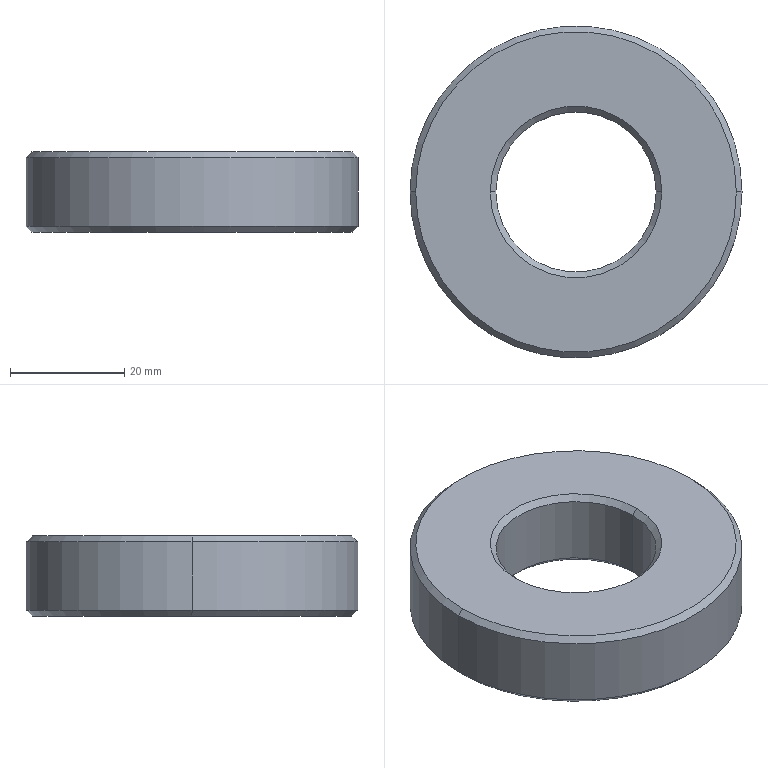Part | STEP file | 1 solid | 14 faces | box 58 x 58 x 14 mm | volume 28098 mm3 | cone 8 | cylinder 4 | plane 2 | commonest cylinder face diameters 28 x2 58 x2
STEP:
#1=CARTESIAN_POINT('',(0.,0.,0.));
#2=DIRECTION('',(0.,0.,1.));
#3=DIRECTION('',(1.,0.,0.));
#4=AXIS2_PLACEMENT_3D('',#1,#2,#3);
#5=CARTESIAN_POINT('',(28.,0.,14.));
#6=VERTEX_POINT('',#5);
#7=CARTESIAN_POINT('',(-28.,0.,14.));
#8=VERTEX_POINT('',#7);
#9=CARTESIAN_POINT('',(0.,0.,14.));
#10=DIRECTION('',(0.,0.,1.));
#11=DIRECTION('',(1.,0.,0.));
#12=AXIS2_PLACEMENT_3D('',#9,#10,#11);
#13=CIRCLE('',#12,28.);
#14=CARTESIAN_POINT('',(0.,0.,14.));
#15=DIRECTION('',(0.,0.,-1.));
#16=DIRECTION('',(-1.,0.,0.));
#17=AXIS2_PLACEMENT_3D('',#14,#15,#16);
#18=CONICAL_SURFACE('',#17,28.,0.7854);
#19=CARTESIAN_POINT('',(3.142,0.));
#20=DIRECTION('',(-1.,0.));
#21=VECTOR('',#20,1.);
#22=LINE('',#19,#21);
#23=(GEOMETRIC_REPRESENTATION_CONTEXT(2)PARAMETRIC_REPRESENTATION_CONTEXT()REPRESENTATION_CONTEXT('',''));
#24=DEFINITIONAL_REPRESENTATION('',(#22),#23);
#25=PCURVE('',#18,#24);
#26=CARTESIAN_POINT('',(0.,0.,14.));
#27=DIRECTION('',(0.,0.,1.));
#28=DIRECTION('',(1.,0.,0.));
#29=AXIS2_PLACEMENT_3D('',#26,#27,#28);
#30=PLANE('',#29);
#31=CARTESIAN_POINT('',(0.,0.));
#32=DIRECTION('',(1.,0.));
#33=AXIS2_PLACEMENT_2D('',#31,#32);
#34=CIRCLE('',#33,28.);
#35=(GEOMETRIC_REPRESENTATION_CONTEXT(2)PARAMETRIC_REPRESENTATION_CONTEXT()REPRESENTATION_CONTEXT('',''));
#36=DEFINITIONAL_REPRESENTATION('',(#34),#35);
#37=PCURVE('',#30,#36);
#38=SURFACE_CURVE('',#13,(#25,#37),.PCURVE_S1.);
#39=EDGE_CURVE('',#6,#8,#38,.T.);
#40=ORIENTED_EDGE('',*,*,#39,.F.);
#41=CARTESIAN_POINT('',(29.,0.,13.));
#42=VERTEX_POINT('',#41);
#43=CARTESIAN_POINT('',(28.,0.,14.));
#44=DIRECTION('',(0.7071,0.,-0.7071));
#45=VECTOR('',#44,1.);
#46=LINE('',#43,#45);
#47=CARTESIAN_POINT('',(3.142,0.));
#48=DIRECTION('',(0.,1.));
#49=VECTOR('',#48,1.);
#50=LINE('',#47,#49);
#51=(GEOMETRIC_REPRESENTATION_CONTEXT(2)PARAMETRIC_REPRESENTATION_CONTEXT()REPRESENTATION_CONTEXT('',''));
#52=DEFINITIONAL_REPRESENTATION('',(#50),#51);
#53=PCURVE('',#18,#52);
#54=CARTESIAN_POINT('',(0.,0.,14.));
#55=DIRECTION('',(0.,0.,-1.));
#56=DIRECTION('',(-1.,0.,0.));
#57=AXIS2_PLACEMENT_3D('',#54,#55,#56);
#58=CONICAL_SURFACE('',#57,28.,0.7854);
#59=CARTESIAN_POINT('',(3.142,0.));
#60=DIRECTION('',(0.,1.));
#61=VECTOR('',#60,1.);
#62=LINE('',#59,#61);
#63=(GEOMETRIC_REPRESENTATION_CONTEXT(2)PARAMETRIC_REPRESENTATION_CONTEXT()REPRESENTATION_CONTEXT('',''));
#64=DEFINITIONAL_REPRESENTATION('',(#62),#63);
#65=PCURVE('',#58,#64);
#66=SURFACE_CURVE('',#46,(#53,#65),.PCURVE_S1.);
#67=EDGE_CURVE('',#6,#42,#66,.T.);
#68=ORIENTED_EDGE('',*,*,#67,.T.);
#69=CARTESIAN_POINT('',(-29.,0.,13.));
#70=VERTEX_POINT('',#69);
#71=CARTESIAN_POINT('',(0.,0.,13.));
#72=DIRECTION('',(0.,0.,-1.));
#73=DIRECTION('',(1.,0.,0.));
#74=AXIS2_PLACEMENT_3D('',#71,#72,#73);
#75=CIRCLE('',#74,29.);
#76=CARTESIAN_POINT('',(-3.142,1.));
#77=DIRECTION('',(1.,0.));
#78=VECTOR('',#77,1.);
#79=LINE('',#76,#78);
#80=(GEOMETRIC_REPRESENTATION_CONTEXT(2)PARAMETRIC_REPRESENTATION_CONTEXT()REPRESENTATION_CONTEXT('',''));
#81=DEFINITIONAL_REPRESENTATION('',(#79),#80);
#82=PCURVE('',#18,#81);
#83=CARTESIAN_POINT('',(0.,0.,14.));
#84=DIRECTION('',(0.,0.,-1.));
#85=DIRECTION('',(-1.,0.,0.));
#86=AXIS2_PLACEMENT_3D('',#83,#84,#85);
#87=CYLINDRICAL_SURFACE('',#86,29.);
#88=CARTESIAN_POINT('',(-3.142,1.));
#89=DIRECTION('',(1.,0.));
#90=VECTOR('',#89,1.);
#91=LINE('',#88,#90);
#92=(GEOMETRIC_REPRESENTATION_CONTEXT(2)PARAMETRIC_REPRESENTATION_CONTEXT()REPRESENTATION_CONTEXT('',''));
#93=DEFINITIONAL_REPRESENTATION('',(#91),#92);
#94=PCURVE('',#87,#93);
#95=SURFACE_CURVE('',#75,(#82,#94),.PCURVE_S1.);
#96=EDGE_CURVE('',#70,#42,#95,.T.);
#97=ORIENTED_EDGE('',*,*,#96,.F.);
#98=CARTESIAN_POINT('',(-28.,0.,14.));
#99=DIRECTION('',(-0.7071,0.,-0.7071));
#100=VECTOR('',#99,1.);
#101=LINE('',#98,#100);
#102=CARTESIAN_POINT('',(0.,0.));
#103=DIRECTION('',(0.,1.));
#104=VECTOR('',#103,1.);
#105=LINE('',#102,#104);
#106=(GEOMETRIC_REPRESENTATION_CONTEXT(2)PARAMETRIC_REPRESENTATION_CONTEXT()REPRESENTATION_CONTEXT('',''));
#107=DEFINITIONAL_REPRESENTATION('',(#105),#106);
#108=PCURVE('',#18,#107);
#109=CARTESIAN_POINT('',(6.283,0.));
#110=DIRECTION('',(0.,1.));
#111=VECTOR('',#110,1.);
#112=LINE('',#109,#111);
#113=(GEOMETRIC_REPRESENTATION_CONTEXT(2)PARAMETRIC_REPRESENTATION_CONTEXT()REPRESENTATION_CONTEXT('',''));
#114=DEFINITIONAL_REPRESENTATION('',(#112),#113);
#115=PCURVE('',#58,#114);
#116=SURFACE_CURVE('',#101,(#108,#115),.PCURVE_S1.);
#117=EDGE_CURVE('',#8,#70,#116,.T.);
#118=ORIENTED_EDGE('',*,*,#117,.F.);
#119=EDGE_LOOP('',(#40,#68,#97,#118));
#120=FACE_BOUND('',#119,.T.);
#121=ADVANCED_FACE('',(#120),#18,.T.);
#122=CARTESIAN_POINT('',(14.,0.,13.));
#123=VERTEX_POINT('',#122);
#124=CARTESIAN_POINT('',(15.,0.,14.));
#125=VERTEX_POINT('',#124);
#126=CARTESIAN_POINT('',(14.,0.,13.));
#127=DIRECTION('',(0.7071,0.,0.7071));
#128=VECTOR('',#127,1.);
#129=LINE('',#126,#128);
#130=CARTESIAN_POINT('',(0.,0.,13.));
#131=DIRECTION('',(0.,0.,1.));
#132=DIRECTION('',(1.,0.,0.));
#133=AXIS2_PLACEMENT_3D('',#130,#131,#132);
#134=CONICAL_SURFACE('',#133,14.,0.7854);
#135=CARTESIAN_POINT('',(6.283,0.));
#136=DIRECTION('',(0.,1.));
#137=VECTOR('',#136,1.);
#138=LINE('',#135,#137);
#139=(GEOMETRIC_REPRESENTATION_CONTEXT(2)PARAMETRIC_REPRESENTATION_CONTEXT()REPRESENTATION_CONTEXT('',''));
#140=DEFINITIONAL_REPRESENTATION('',(#138),#139);
#141=PCURVE('',#134,#140);
#142=CARTESIAN_POINT('',(0.,0.,13.));
#143=DIRECTION('',(0.,0.,1.));
#144=DIRECTION('',(1.,0.,0.));
#145=AXIS2_PLACEMENT_3D('',#142,#143,#144);
#146=CONICAL_SURFACE('',#145,14.,0.7854);
#147=CARTESIAN_POINT('',(0.,0.));
#148=DIRECTION('',(0.,1.));
#149=VECTOR('',#148,1.);
#150=LINE('',#147,#149);
#151=(GEOMETRIC_REPRESENTATION_CONTEXT(2)PARAMETRIC_REPRESENTATION_CONTEXT()REPRESENTATION_CONTEXT('',''));
#152=DEFINITIONAL_REPRESENTATION('',(#150),#151);
#153=PCURVE('',#146,#152);
#154=SURFACE_CURVE('',#129,(#141,#153),.PCURVE_S1.);
#155=EDGE_CURVE('',#123,#125,#154,.T.);
#156=ORIENTED_EDGE('',*,*,#155,.T.);
#157=CARTESIAN_POINT('',(-15.,0.,14.));
#158=VERTEX_POINT('',#157);
#159=CARTESIAN_POINT('',(0.,0.,14.));
#160=DIRECTION('',(0.,0.,-1.));
#161=DIRECTION('',(1.,0.,0.));
#162=AXIS2_PLACEMENT_3D('',#159,#160,#161);
#163=CIRCLE('',#162,15.);
#164=CARTESIAN_POINT('',(6.283,1.));
#165=DIRECTION('',(-1.,0.));
#166=VECTOR('',#165,1.);
#167=LINE('',#164,#166);
#168=(GEOMETRIC_REPRESENTATION_CONTEXT(2)PARAMETRIC_REPRESENTATION_CONTEXT()REPRESENTATION_CONTEXT('',''));
#169=DEFINITIONAL_REPRESENTATION('',(#167),#168);
#170=PCURVE('',#134,#169);
#171=CARTESIAN_POINT('',(15.,0.));
#172=CARTESIAN_POINT('',(15.,-25.981));
#173=CARTESIAN_POINT('',(-7.5,-12.99));
#174=CARTESIAN_POINT('',(-30.,0.));
#175=CARTESIAN_POINT('',(-7.5,12.99));
#176=CARTESIAN_POINT('',(15.,25.981));
#177=CARTESIAN_POINT('',(15.,0.));
#178=(BOUNDED_CURVE()B_SPLINE_CURVE(2,(#171,#172,#173,#174,#175,#176,#177),.UNSPECIFIED.,.T.,.F.)B_SPLINE_CURVE_WITH_KNOTS((1,2,2,2,2,1),(-2.094,0.,2.094,4.189,6.283,8.378),.UNSPECIFIED.)CURVE()GEOMETRIC_REPRESENTATION_ITEM()RATIONAL_B_SPLINE_CURVE((1.,0.5,1.,0.5,1.,0.5,1.))REPRESENTATION_ITEM(''));
#179=(GEOMETRIC_REPRESENTATION_CONTEXT(2)PARAMETRIC_REPRESENTATION_CONTEXT()REPRESENTATION_CONTEXT('',''));
#180=DEFINITIONAL_REPRESENTATION('',(#178),#179);
#181=PCURVE('',#30,#180);
#182=SURFACE_CURVE('',#163,(#170,#181),.PCURVE_S1.);
#183=EDGE_CURVE('',#125,#158,#182,.T.);
#184=ORIENTED_EDGE('',*,*,#183,.T.);
#185=CARTESIAN_POINT('',(-14.,0.,13.));
#186=VERTEX_POINT('',#185);
#187=CARTESIAN_POINT('',(-14.,0.,13.));
#188=DIRECTION('',(-0.7071,0.,0.7071));
#189=VECTOR('',#188,1.);
#190=LINE('',#187,#189);
#191=CARTESIAN_POINT('',(3.142,0.));
#192=DIRECTION('',(0.,1.));
#193=VECTOR('',#192,1.);
#194=LINE('',#191,#193);
#195=(GEOMETRIC_REPRESENTATION_CONTEXT(2)PARAMETRIC_REPRESENTATION_CONTEXT()REPRESENTATION_CONTEXT('',''));
#196=DEFINITIONAL_REPRESENTATION('',(#194),#195);
#197=PCURVE('',#134,#196);
#198=CARTESIAN_POINT('',(3.142,0.));
#199=DIRECTION('',(0.,1.));
#200=VECTOR('',#199,1.);
#201=LINE('',#198,#200);
#202=(GEOMETRIC_REPRESENTATION_CONTEXT(2)PARAMETRIC_REPRESENTATION_CONTEXT()REPRESENTATION_CONTEXT('',''));
#203=DEFINITIONAL_REPRESENTATION('',(#201),#202);
#204=PCURVE('',#146,#203);
#205=SURFACE_CURVE('',#190,(#197,#204),.PCURVE_S1.);
#206=EDGE_CURVE('',#186,#158,#205,.T.);
#207=ORIENTED_EDGE('',*,*,#206,.F.);
#208=CARTESIAN_POINT('',(0.,0.,13.));
#209=DIRECTION('',(0.,0.,1.));
#210=DIRECTION('',(1.,0.,0.));
#211=AXIS2_PLACEMENT_3D('',#208,#209,#210);
#212=CIRCLE('',#211,14.);
#213=CARTESIAN_POINT('',(0.,0.));
#214=DIRECTION('',(1.,0.));
#215=VECTOR('',#214,1.);
#216=LINE('',#213,#215);
#217=(GEOMETRIC_REPRESENTATION_CONTEXT(2)PARAMETRIC_REPRESENTATION_CONTEXT()REPRESENTATION_CONTEXT('',''));
#218=DEFINITIONAL_REPRESENTATION('',(#216),#217);
#219=PCURVE('',#134,#218);
#220=CARTESIAN_POINT('',(0.,0.,14.));
#221=DIRECTION('',(0.,0.,-1.));
#222=DIRECTION('',(-1.,0.,0.));
#223=AXIS2_PLACEMENT_3D('',#220,#221,#222);
#224=CYLINDRICAL_SURFACE('',#223,14.);
#225=CARTESIAN_POINT('',(9.425,1.));
#226=DIRECTION('',(-1.,0.));
#227=VECTOR('',#226,1.);
#228=LINE('',#225,#227);
#229=(GEOMETRIC_REPRESENTATION_CONTEXT(2)PARAMETRIC_REPRESENTATION_CONTEXT()REPRESENTATION_CONTEXT('',''));
#230=DEFINITIONAL_REPRESENTATION('',(#228),#229);
#231=PCURVE('',#224,#230);
#232=SURFACE_CURVE('',#212,(#219,#231),.PCURVE_S1.);
#233=EDGE_CURVE('',#186,#123,#232,.T.);
#234=ORIENTED_EDGE('',*,*,#233,.T.);
#235=EDGE_LOOP('',(#156,#184,#207,#234));
#236=FACE_BOUND('',#235,.F.);
#237=ADVANCED_FACE('',(#236),#134,.F.);
#238=CARTESIAN_POINT('',(-28.,0.,0.));
#239=VERTEX_POINT('',#238);
#240=CARTESIAN_POINT('',(28.,0.,0.));
#241=VERTEX_POINT('',#240);
#242=CARTESIAN_POINT('',(0.,0.,0.));
#243=DIRECTION('',(0.,0.,-1.));
#244=DIRECTION('',(1.,0.,0.));
#245=AXIS2_PLACEMENT_3D('',#242,#243,#244);
#246=CIRCLE('',#245,28.);
#247=CARTESIAN_POINT('',(0.,0.,1.));
#248=DIRECTION('',(0.,0.,1.));
#249=DIRECTION('',(1.,0.,0.));
#250=AXIS2_PLACEMENT_3D('',#247,#248,#249);
#251=CONICAL_SURFACE('',#250,29.,0.7854);
#252=CARTESIAN_POINT('',(6.283,-1.));
#253=DIRECTION('',(-1.,0.));
#254=VECTOR('',#253,1.);
#255=LINE('',#252,#254);
#256=(GEOMETRIC_REPRESENTATION_CONTEXT(2)PARAMETRIC_REPRESENTATION_CONTEXT()REPRESENTATION_CONTEXT('',''));
#257=DEFINITIONAL_REPRESENTATION('',(#255),#256);
#258=PCURVE('',#251,#257);
#259=CARTESIAN_POINT('',(0.,0.,0.));
#260=DIRECTION('',(0.,0.,1.));
#261=DIRECTION('',(1.,0.,0.));
#262=AXIS2_PLACEMENT_3D('',#259,#260,#261);
#263=PLANE('',#262);
#264=CARTESIAN_POINT('',(28.,0.));
#265=CARTESIAN_POINT('',(28.,-48.497));
#266=CARTESIAN_POINT('',(-14.,-24.249));
#267=CARTESIAN_POINT('',(-56.,0.));
#268=CARTESIAN_POINT('',(-14.,24.249));
#269=CARTESIAN_POINT('',(28.,48.497));
#270=CARTESIAN_POINT('',(28.,0.));
#271=(BOUNDED_CURVE()B_SPLINE_CURVE(2,(#264,#265,#266,#267,#268,#269,#270),.UNSPECIFIED.,.T.,.F.)B_SPLINE_CURVE_WITH_KNOTS((1,2,2,2,2,1),(-2.094,0.,2.094,4.189,6.283,8.378),.UNSPECIFIED.)CURVE()GEOMETRIC_REPRESENTATION_ITEM()RATIONAL_B_SPLINE_CURVE((1.,0.5,1.,0.5,1.,0.5,1.))REPRESENTATION_ITEM(''));
#272=(GEOMETRIC_REPRESENTATION_CONTEXT(2)PARAMETRIC_REPRESENTATION_CONTEXT()REPRESENTATION_CONTEXT('',''));
#273=DEFINITIONAL_REPRESENTATION('',(#271),#272);
#274=PCURVE('',#263,#273);
#275=SURFACE_CURVE('',#246,(#258,#274),.PCURVE_S1.);
#276=EDGE_CURVE('',#239,#241,#275,.T.);
#277=ORIENTED_EDGE('',*,*,#276,.F.);
#278=CARTESIAN_POINT('',(-29.,0.,1.));
#279=VERTEX_POINT('',#278);
#280=CARTESIAN_POINT('',(-29.,0.,1.));
#281=DIRECTION('',(-0.7071,0.,0.7071));
#282=VECTOR('',#281,1.);
#283=LINE('',#280,#282);
#284=CARTESIAN_POINT('',(3.142,0.));
#285=DIRECTION('',(0.,1.));
#286=VECTOR('',#285,1.);
#287=LINE('',#284,#286);
#288=(GEOMETRIC_REPRESENTATION_CONTEXT(2)PARAMETRIC_REPRESENTATION_CONTEXT()REPRESENTATION_CONTEXT('',''));
#289=DEFINITIONAL_REPRESENTATION('',(#287),#288);
#290=PCURVE('',#251,#289);
#291=CARTESIAN_POINT('',(0.,0.,1.));
#292=DIRECTION('',(0.,0.,1.));
#293=DIRECTION('',(1.,0.,0.));
#294=AXIS2_PLACEMENT_3D('',#291,#292,#293);
#295=CONICAL_SURFACE('',#294,29.,0.7854);
#296=CARTESIAN_POINT('',(3.142,0.));
#297=DIRECTION('',(0.,1.));
#298=VECTOR('',#297,1.);
#299=LINE('',#296,#298);
#300=(GEOMETRIC_REPRESENTATION_CONTEXT(2)PARAMETRIC_REPRESENTATION_CONTEXT()REPRESENTATION_CONTEXT('',''));
#301=DEFINITIONAL_REPRESENTATION('',(#299),#300);
#302=PCURVE('',#295,#301);
#303=SURFACE_CURVE('',#283,(#290,#302),.PCURVE_S1.);
#304=EDGE_CURVE('',#239,#279,#303,.T.);
#305=ORIENTED_EDGE('',*,*,#304,.T.);
#306=CARTESIAN_POINT('',(29.,0.,1.));
#307=VERTEX_POINT('',#306);
#308=CARTESIAN_POINT('',(0.,0.,1.));
#309=DIRECTION('',(0.,0.,1.));
#310=DIRECTION('',(1.,0.,0.));
#311=AXIS2_PLACEMENT_3D('',#308,#309,#310);
#312=CIRCLE('',#311,29.);
#313=CARTESIAN_POINT('',(0.,0.));
#314=DIRECTION('',(1.,0.));
#315=VECTOR('',#314,1.);
#316=LINE('',#313,#315);
#317=(GEOMETRIC_REPRESENTATION_CONTEXT(2)PARAMETRIC_REPRESENTATION_CONTEXT()REPRESENTATION_CONTEXT('',''));
#318=DEFINITIONAL_REPRESENTATION('',(#316),#317);
#319=PCURVE('',#251,#318);
#320=CARTESIAN_POINT('',(3.142,13.));
#321=DIRECTION('',(-1.,0.));
#322=VECTOR('',#321,1.);
#323=LINE('',#320,#322);
#324=(GEOMETRIC_REPRESENTATION_CONTEXT(2)PARAMETRIC_REPRESENTATION_CONTEXT()REPRESENTATION_CONTEXT('',''));
#325=DEFINITIONAL_REPRESENTATION('',(#323),#324);
#326=PCURVE('',#87,#325);
#327=SURFACE_CURVE('',#312,(#319,#326),.PCURVE_S1.);
#328=EDGE_CURVE('',#307,#279,#327,.T.);
#329=ORIENTED_EDGE('',*,*,#328,.F.);
#330=CARTESIAN_POINT('',(29.,0.,1.));
#331=DIRECTION('',(0.7071,0.,0.7071));
#332=VECTOR('',#331,1.);
#333=LINE('',#330,#332);
#334=CARTESIAN_POINT('',(0.,0.));
#335=DIRECTION('',(0.,1.));
#336=VECTOR('',#335,1.);
#337=LINE('',#334,#336);
#338=(GEOMETRIC_REPRESENTATION_CONTEXT(2)PARAMETRIC_REPRESENTATION_CONTEXT()REPRESENTATION_CONTEXT('',''));
#339=DEFINITIONAL_REPRESENTATION('',(#337),#338);
#340=PCURVE('',#251,#339);
#341=CARTESIAN_POINT('',(6.283,0.));
#342=DIRECTION('',(0.,1.));
#343=VECTOR('',#342,1.);
#344=LINE('',#341,#343);
#345=(GEOMETRIC_REPRESENTATION_CONTEXT(2)PARAMETRIC_REPRESENTATION_CONTEXT()REPRESENTATION_CONTEXT('',''));
#346=DEFINITIONAL_REPRESENTATION('',(#344),#345);
#347=PCURVE('',#295,#346);
#348=SURFACE_CURVE('',#333,(#340,#347),.PCURVE_S1.);
#349=EDGE_CURVE('',#241,#307,#348,.T.);
#350=ORIENTED_EDGE('',*,*,#349,.F.);
#351=EDGE_LOOP('',(#277,#305,#329,#350));
#352=FACE_BOUND('',#351,.T.);
#353=ADVANCED_FACE('',(#352),#251,.T.);
#354=CARTESIAN_POINT('',(-14.,0.,1.));
#355=VERTEX_POINT('',#354);
#356=CARTESIAN_POINT('',(-15.,0.,0.));
#357=VERTEX_POINT('',#356);
#358=CARTESIAN_POINT('',(-15.,0.,0.));
#359=DIRECTION('',(-0.7071,0.,-0.7071));
#360=VECTOR('',#359,1.);
#361=LINE('',#358,#360);
#362=CARTESIAN_POINT('',(0.,0.,0.));
#363=DIRECTION('',(0.,0.,-1.));
#364=DIRECTION('',(-1.,0.,0.));
#365=AXIS2_PLACEMENT_3D('',#362,#363,#364);
#366=CONICAL_SURFACE('',#365,15.,0.7854);
#367=CARTESIAN_POINT('',(6.283,0.));
#368=DIRECTION('',(0.,1.));
#369=VECTOR('',#368,1.);
#370=LINE('',#367,#369);
#371=(GEOMETRIC_REPRESENTATION_CONTEXT(2)PARAMETRIC_REPRESENTATION_CONTEXT()REPRESENTATION_CONTEXT('',''));
#372=DEFINITIONAL_REPRESENTATION('',(#370),#371);
#373=PCURVE('',#366,#372);
#374=CARTESIAN_POINT('',(0.,0.,0.));
#375=DIRECTION('',(0.,0.,-1.));
#376=DIRECTION('',(-1.,0.,0.));
#377=AXIS2_PLACEMENT_3D('',#374,#375,#376);
#378=CONICAL_SURFACE('',#377,15.,0.7854);
#379=CARTESIAN_POINT('',(0.,0.));
#380=DIRECTION('',(0.,1.));
#381=VECTOR('',#380,1.);
#382=LINE('',#379,#381);
#383=(GEOMETRIC_REPRESENTATION_CONTEXT(2)PARAMETRIC_REPRESENTATION_CONTEXT()REPRESENTATION_CONTEXT('',''));
#384=DEFINITIONAL_REPRESENTATION('',(#382),#383);
#385=PCURVE('',#378,#384);
#386=SURFACE_CURVE('',#361,(#373,#385),.PCURVE_S1.);
#387=EDGE_CURVE('',#355,#357,#386,.T.);
#388=ORIENTED_EDGE('',*,*,#387,.T.);
#389=CARTESIAN_POINT('',(15.,0.,0.));
#390=VERTEX_POINT('',#389);
#391=CARTESIAN_POINT('',(0.,0.,0.));
#392=DIRECTION('',(0.,0.,1.));
#393=DIRECTION('',(1.,0.,0.));
#394=AXIS2_PLACEMENT_3D('',#391,#392,#393);
#395=CIRCLE('',#394,15.);
#396=CARTESIAN_POINT('',(9.425,0.));
#397=DIRECTION('',(-1.,0.));
#398=VECTOR('',#397,1.);
#399=LINE('',#396,#398);
#400=(GEOMETRIC_REPRESENTATION_CONTEXT(2)PARAMETRIC_REPRESENTATION_CONTEXT()REPRESENTATION_CONTEXT('',''));
#401=DEFINITIONAL_REPRESENTATION('',(#399),#400);
#402=PCURVE('',#366,#401);
#403=CARTESIAN_POINT('',(0.,0.));
#404=DIRECTION('',(1.,0.));
#405=AXIS2_PLACEMENT_2D('',#403,#404);
#406=CIRCLE('',#405,15.);
#407=(GEOMETRIC_REPRESENTATION_CONTEXT(2)PARAMETRIC_REPRESENTATION_CONTEXT()REPRESENTATION_CONTEXT('',''));
#408=DEFINITIONAL_REPRESENTATION('',(#406),#407);
#409=PCURVE('',#263,#408);
#410=SURFACE_CURVE('',#395,(#402,#409),.PCURVE_S1.);
#411=EDGE_CURVE('',#357,#390,#410,.T.);
#412=ORIENTED_EDGE('',*,*,#411,.T.);
#413=CARTESIAN_POINT('',(14.,0.,1.));
#414=VERTEX_POINT('',#413);
#415=CARTESIAN_POINT('',(15.,0.,0.));
#416=DIRECTION('',(0.7071,0.,-0.7071));
#417=VECTOR('',#416,1.);
#418=LINE('',#415,#417);
#419=CARTESIAN_POINT('',(3.142,0.));
#420=DIRECTION('',(0.,1.));
#421=VECTOR('',#420,1.);
#422=LINE('',#419,#421);
#423=(GEOMETRIC_REPRESENTATION_CONTEXT(2)PARAMETRIC_REPRESENTATION_CONTEXT()REPRESENTATION_CONTEXT('',''));
#424=DEFINITIONAL_REPRESENTATION('',(#422),#423);
#425=PCURVE('',#366,#424);
#426=CARTESIAN_POINT('',(3.142,0.));
#427=DIRECTION('',(0.,1.));
#428=VECTOR('',#427,1.);
#429=LINE('',#426,#428);
#430=(GEOMETRIC_REPRESENTATION_CONTEXT(2)PARAMETRIC_REPRESENTATION_CONTEXT()REPRESENTATION_CONTEXT('',''));
#431=DEFINITIONAL_REPRESENTATION('',(#429),#430);
#432=PCURVE('',#378,#431);
#433=SURFACE_CURVE('',#418,(#425,#432),.PCURVE_S1.);
#434=EDGE_CURVE('',#414,#390,#433,.T.);
#435=ORIENTED_EDGE('',*,*,#434,.F.);
#436=CARTESIAN_POINT('',(0.,0.,1.));
#437=DIRECTION('',(0.,0.,-1.));
#438=DIRECTION('',(1.,0.,0.));
#439=AXIS2_PLACEMENT_3D('',#436,#437,#438);
#440=CIRCLE('',#439,14.);
#441=CARTESIAN_POINT('',(3.142,-1.));
#442=DIRECTION('',(1.,0.));
#443=VECTOR('',#442,1.);
#444=LINE('',#441,#443);
#445=(GEOMETRIC_REPRESENTATION_CONTEXT(2)PARAMETRIC_REPRESENTATION_CONTEXT()REPRESENTATION_CONTEXT('',''));
#446=DEFINITIONAL_REPRESENTATION('',(#444),#445);
#447=PCURVE('',#366,#446);
#448=CARTESIAN_POINT('',(3.142,13.));
#449=DIRECTION('',(1.,0.));
#450=VECTOR('',#449,1.);
#451=LINE('',#448,#450);
#452=(GEOMETRIC_REPRESENTATION_CONTEXT(2)PARAMETRIC_REPRESENTATION_CONTEXT()REPRESENTATION_CONTEXT('',''));
#453=DEFINITIONAL_REPRESENTATION('',(#451),#452);
#454=PCURVE('',#224,#453);
#455=SURFACE_CURVE('',#440,(#447,#454),.PCURVE_S1.);
#456=EDGE_CURVE('',#414,#355,#455,.T.);
#457=ORIENTED_EDGE('',*,*,#456,.T.);
#458=EDGE_LOOP('',(#388,#412,#435,#457));
#459=FACE_BOUND('',#458,.F.);
#460=ADVANCED_FACE('',(#459),#366,.F.);
#461=CARTESIAN_POINT('',(-14.,0.,14.));
#462=DIRECTION('',(0.,0.,-1.));
#463=VECTOR('',#462,1.);
#464=LINE('',#461,#463);
#465=CARTESIAN_POINT('',(6.283,0.));
#466=DIRECTION('',(0.,1.));
#467=VECTOR('',#466,1.);
#468=LINE('',#465,#467);
#469=(GEOMETRIC_REPRESENTATION_CONTEXT(2)PARAMETRIC_REPRESENTATION_CONTEXT()REPRESENTATION_CONTEXT('',''));
#470=DEFINITIONAL_REPRESENTATION('',(#468),#469);
#471=PCURVE('',#224,#470);
#472=CARTESIAN_POINT('',(0.,0.,14.));
#473=DIRECTION('',(0.,0.,-1.));
#474=DIRECTION('',(-1.,0.,0.));
#475=AXIS2_PLACEMENT_3D('',#472,#473,#474);
#476=CYLINDRICAL_SURFACE('',#475,14.);
#477=CARTESIAN_POINT('',(0.,0.));
#478=DIRECTION('',(0.,1.));
#479=VECTOR('',#478,1.);
#480=LINE('',#477,#479);
#481=(GEOMETRIC_REPRESENTATION_CONTEXT(2)PARAMETRIC_REPRESENTATION_CONTEXT()REPRESENTATION_CONTEXT('',''));
#482=DEFINITIONAL_REPRESENTATION('',(#480),#481);
#483=PCURVE('',#476,#482);
#484=SURFACE_CURVE('',#464,(#471,#483),.PCURVE_S1.);
#485=EDGE_CURVE('',#186,#355,#484,.T.);
#486=ORIENTED_EDGE('',*,*,#485,.T.);
#487=ORIENTED_EDGE('',*,*,#456,.F.);
#488=CARTESIAN_POINT('',(14.,0.,14.));
#489=DIRECTION('',(0.,0.,-1.));
#490=VECTOR('',#489,1.);
#491=LINE('',#488,#490);
#492=CARTESIAN_POINT('',(3.142,0.));
#493=DIRECTION('',(0.,1.));
#494=VECTOR('',#493,1.);
#495=LINE('',#492,#494);
#496=(GEOMETRIC_REPRESENTATION_CONTEXT(2)PARAMETRIC_REPRESENTATION_CONTEXT()REPRESENTATION_CONTEXT('',''));
#497=DEFINITIONAL_REPRESENTATION('',(#495),#496);
#498=PCURVE('',#224,#497);
#499=CARTESIAN_POINT('',(3.142,0.));
#500=DIRECTION('',(0.,1.));
#501=VECTOR('',#500,1.);
#502=LINE('',#499,#501);
#503=(GEOMETRIC_REPRESENTATION_CONTEXT(2)PARAMETRIC_REPRESENTATION_CONTEXT()REPRESENTATION_CONTEXT('',''));
#504=DEFINITIONAL_REPRESENTATION('',(#502),#503);
#505=PCURVE('',#476,#504);
#506=SURFACE_CURVE('',#491,(#498,#505),.PCURVE_S1.);
#507=EDGE_CURVE('',#123,#414,#506,.T.);
#508=ORIENTED_EDGE('',*,*,#507,.F.);
#509=ORIENTED_EDGE('',*,*,#233,.F.);
#510=EDGE_LOOP('',(#486,#487,#508,#509));
#511=FACE_BOUND('',#510,.F.);
#512=ADVANCED_FACE('',(#511),#224,.F.);
#513=ORIENTED_EDGE('',*,*,#96,.T.);
#514=CARTESIAN_POINT('',(29.,0.,14.));
#515=DIRECTION('',(0.,0.,-1.));
#516=VECTOR('',#515,1.);
#517=LINE('',#514,#516);
#518=CARTESIAN_POINT('',(3.142,0.));
#519=DIRECTION('',(0.,1.));
#520=VECTOR('',#519,1.);
#521=LINE('',#518,#520);
#522=(GEOMETRIC_REPRESENTATION_CONTEXT(2)PARAMETRIC_REPRESENTATION_CONTEXT()REPRESENTATION_CONTEXT('',''));
#523=DEFINITIONAL_REPRESENTATION('',(#521),#522);
#524=PCURVE('',#87,#523);
#525=CARTESIAN_POINT('',(0.,0.,14.));
#526=DIRECTION('',(0.,0.,-1.));
#527=DIRECTION('',(-1.,0.,0.));
#528=AXIS2_PLACEMENT_3D('',#525,#526,#527);
#529=CYLINDRICAL_SURFACE('',#528,29.);
#530=CARTESIAN_POINT('',(3.142,0.));
#531=DIRECTION('',(0.,1.));
#532=VECTOR('',#531,1.);
#533=LINE('',#530,#532);
#534=(GEOMETRIC_REPRESENTATION_CONTEXT(2)PARAMETRIC_REPRESENTATION_CONTEXT()REPRESENTATION_CONTEXT('',''));
#535=DEFINITIONAL_REPRESENTATION('',(#533),#534);
#536=PCURVE('',#529,#535);
#537=SURFACE_CURVE('',#517,(#524,#536),.PCURVE_S1.);
#538=EDGE_CURVE('',#42,#307,#537,.T.);
#539=ORIENTED_EDGE('',*,*,#538,.T.);
#540=ORIENTED_EDGE('',*,*,#328,.T.);
#541=CARTESIAN_POINT('',(-29.,0.,14.));
#542=DIRECTION('',(0.,0.,-1.));
#543=VECTOR('',#542,1.);
#544=LINE('',#541,#543);
#545=CARTESIAN_POINT('',(0.,0.));
#546=DIRECTION('',(0.,1.));
#547=VECTOR('',#546,1.);
#548=LINE('',#545,#547);
#549=(GEOMETRIC_REPRESENTATION_CONTEXT(2)PARAMETRIC_REPRESENTATION_CONTEXT()REPRESENTATION_CONTEXT('',''));
#550=DEFINITIONAL_REPRESENTATION('',(#548),#549);
#551=PCURVE('',#87,#550);
#552=CARTESIAN_POINT('',(6.283,0.));
#553=DIRECTION('',(0.,1.));
#554=VECTOR('',#553,1.);
#555=LINE('',#552,#554);
#556=(GEOMETRIC_REPRESENTATION_CONTEXT(2)PARAMETRIC_REPRESENTATION_CONTEXT()REPRESENTATION_CONTEXT('',''));
#557=DEFINITIONAL_REPRESENTATION('',(#555),#556);
#558=PCURVE('',#529,#557);
#559=SURFACE_CURVE('',#544,(#551,#558),.PCURVE_S1.);
#560=EDGE_CURVE('',#70,#279,#559,.T.);
#561=ORIENTED_EDGE('',*,*,#560,.F.);
#562=EDGE_LOOP('',(#513,#539,#540,#561));
#563=FACE_BOUND('',#562,.T.);
#564=ADVANCED_FACE('',(#563),#87,.T.);
#565=ORIENTED_EDGE('',*,*,#183,.T.);
#566=CARTESIAN_POINT('',(0.,0.,14.));
#567=DIRECTION('',(0.,0.,-1.));
#568=DIRECTION('',(1.,0.,0.));
#569=AXIS2_PLACEMENT_3D('',#566,#567,#568);
#570=CIRCLE('',#569,15.);
#571=CARTESIAN_POINT('',(15.,0.));
#572=CARTESIAN_POINT('',(15.,-25.981));
#573=CARTESIAN_POINT('',(-7.5,-12.99));
#574=CARTESIAN_POINT('',(-30.,0.));
#575=CARTESIAN_POINT('',(-7.5,12.99));
#576=CARTESIAN_POINT('',(15.,25.981));
#577=CARTESIAN_POINT('',(15.,0.));
#578=(BOUNDED_CURVE()B_SPLINE_CURVE(2,(#571,#572,#573,#574,#575,#576,#577),.UNSPECIFIED.,.T.,.F.)B_SPLINE_CURVE_WITH_KNOTS((1,2,2,2,2,1),(-2.094,0.,2.094,4.189,6.283,8.378),.UNSPECIFIED.)CURVE()GEOMETRIC_REPRESENTATION_ITEM()RATIONAL_B_SPLINE_CURVE((1.,0.5,1.,0.5,1.,0.5,1.))REPRESENTATION_ITEM(''));
#579=(GEOMETRIC_REPRESENTATION_CONTEXT(2)PARAMETRIC_REPRESENTATION_CONTEXT()REPRESENTATION_CONTEXT('',''));
#580=DEFINITIONAL_REPRESENTATION('',(#578),#579);
#581=PCURVE('',#30,#580);
#582=CARTESIAN_POINT('',(6.283,1.));
#583=DIRECTION('',(-1.,0.));
#584=VECTOR('',#583,1.);
#585=LINE('',#582,#584);
#586=(GEOMETRIC_REPRESENTATION_CONTEXT(2)PARAMETRIC_REPRESENTATION_CONTEXT()REPRESENTATION_CONTEXT('',''));
#587=DEFINITIONAL_REPRESENTATION('',(#585),#586);
#588=PCURVE('',#146,#587);
#589=SURFACE_CURVE('',#570,(#581,#588),.PCURVE_S1.);
#590=EDGE_CURVE('',#158,#125,#589,.T.);
#591=ORIENTED_EDGE('',*,*,#590,.T.);
#592=EDGE_LOOP('',(#565,#591));
#593=FACE_BOUND('',#592,.T.);
#594=CARTESIAN_POINT('',(0.,0.,14.));
#595=DIRECTION('',(0.,0.,1.));
#596=DIRECTION('',(1.,0.,0.));
#597=AXIS2_PLACEMENT_3D('',#594,#595,#596);
#598=CIRCLE('',#597,28.);
#599=CARTESIAN_POINT('',(0.,0.));
#600=DIRECTION('',(1.,0.));
#601=AXIS2_PLACEMENT_2D('',#599,#600);
#602=CIRCLE('',#601,28.);
#603=(GEOMETRIC_REPRESENTATION_CONTEXT(2)PARAMETRIC_REPRESENTATION_CONTEXT()REPRESENTATION_CONTEXT('',''));
#604=DEFINITIONAL_REPRESENTATION('',(#602),#603);
#605=PCURVE('',#30,#604);
#606=CARTESIAN_POINT('',(9.425,0.));
#607=DIRECTION('',(-1.,0.));
#608=VECTOR('',#607,1.);
#609=LINE('',#606,#608);
#610=(GEOMETRIC_REPRESENTATION_CONTEXT(2)PARAMETRIC_REPRESENTATION_CONTEXT()REPRESENTATION_CONTEXT('',''));
#611=DEFINITIONAL_REPRESENTATION('',(#609),#610);
#612=PCURVE('',#58,#611);
#613=SURFACE_CURVE('',#598,(#605,#612),.PCURVE_S1.);
#614=EDGE_CURVE('',#8,#6,#613,.T.);
#615=ORIENTED_EDGE('',*,*,#614,.T.);
#616=ORIENTED_EDGE('',*,*,#39,.T.);
#617=EDGE_LOOP('',(#615,#616));
#618=FACE_BOUND('',#617,.T.);
#619=ADVANCED_FACE('',(#593,#618),#30,.T.);
#620=ORIENTED_EDGE('',*,*,#411,.T.);
#621=CARTESIAN_POINT('',(0.,0.,0.));
#622=DIRECTION('',(0.,0.,1.));
#623=DIRECTION('',(1.,0.,0.));
#624=AXIS2_PLACEMENT_3D('',#621,#622,#623);
#625=CIRCLE('',#624,15.);
#626=CARTESIAN_POINT('',(0.,0.));
#627=DIRECTION('',(1.,0.));
#628=AXIS2_PLACEMENT_2D('',#626,#627);
#629=CIRCLE('',#628,15.);
#630=(GEOMETRIC_REPRESENTATION_CONTEXT(2)PARAMETRIC_REPRESENTATION_CONTEXT()REPRESENTATION_CONTEXT('',''));
#631=DEFINITIONAL_REPRESENTATION('',(#629),#630);
#632=PCURVE('',#263,#631);
#633=CARTESIAN_POINT('',(3.142,0.));
#634=DIRECTION('',(-1.,0.));
#635=VECTOR('',#634,1.);
#636=LINE('',#633,#635);
#637=(GEOMETRIC_REPRESENTATION_CONTEXT(2)PARAMETRIC_REPRESENTATION_CONTEXT()REPRESENTATION_CONTEXT('',''));
#638=DEFINITIONAL_REPRESENTATION('',(#636),#637);
#639=PCURVE('',#378,#638);
#640=SURFACE_CURVE('',#625,(#632,#639),.PCURVE_S1.);
#641=EDGE_CURVE('',#390,#357,#640,.T.);
#642=ORIENTED_EDGE('',*,*,#641,.T.);
#643=EDGE_LOOP('',(#620,#642));
#644=FACE_BOUND('',#643,.T.);
#645=CARTESIAN_POINT('',(0.,0.,0.));
#646=DIRECTION('',(0.,0.,-1.));
#647=DIRECTION('',(1.,0.,0.));
#648=AXIS2_PLACEMENT_3D('',#645,#646,#647);
#649=CIRCLE('',#648,28.);
#650=CARTESIAN_POINT('',(28.,0.));
#651=CARTESIAN_POINT('',(28.,-48.497));
#652=CARTESIAN_POINT('',(-14.,-24.249));
#653=CARTESIAN_POINT('',(-56.,0.));
#654=CARTESIAN_POINT('',(-14.,24.249));
#655=CARTESIAN_POINT('',(28.,48.497));
#656=CARTESIAN_POINT('',(28.,0.));
#657=(BOUNDED_CURVE()B_SPLINE_CURVE(2,(#650,#651,#652,#653,#654,#655,#656),.UNSPECIFIED.,.T.,.F.)B_SPLINE_CURVE_WITH_KNOTS((1,2,2,2,2,1),(-2.094,0.,2.094,4.189,6.283,8.378),.UNSPECIFIED.)CURVE()GEOMETRIC_REPRESENTATION_ITEM()RATIONAL_B_SPLINE_CURVE((1.,0.5,1.,0.5,1.,0.5,1.))REPRESENTATION_ITEM(''));
#658=(GEOMETRIC_REPRESENTATION_CONTEXT(2)PARAMETRIC_REPRESENTATION_CONTEXT()REPRESENTATION_CONTEXT('',''));
#659=DEFINITIONAL_REPRESENTATION('',(#657),#658);
#660=PCURVE('',#263,#659);
#661=CARTESIAN_POINT('',(6.283,-1.));
#662=DIRECTION('',(-1.,0.));
#663=VECTOR('',#662,1.);
#664=LINE('',#661,#663);
#665=(GEOMETRIC_REPRESENTATION_CONTEXT(2)PARAMETRIC_REPRESENTATION_CONTEXT()REPRESENTATION_CONTEXT('',''));
#666=DEFINITIONAL_REPRESENTATION('',(#664),#665);
#667=PCURVE('',#295,#666);
#668=SURFACE_CURVE('',#649,(#660,#667),.PCURVE_S1.);
#669=EDGE_CURVE('',#241,#239,#668,.T.);
#670=ORIENTED_EDGE('',*,*,#669,.T.);
#671=ORIENTED_EDGE('',*,*,#276,.T.);
#672=EDGE_LOOP('',(#670,#671));
#673=FACE_BOUND('',#672,.T.);
#674=ADVANCED_FACE('',(#644,#673),#263,.F.);
#675=ORIENTED_EDGE('',*,*,#538,.F.);
#676=CARTESIAN_POINT('',(0.,0.,13.));
#677=DIRECTION('',(0.,0.,-1.));
#678=DIRECTION('',(1.,0.,0.));
#679=AXIS2_PLACEMENT_3D('',#676,#677,#678);
#680=CIRCLE('',#679,29.);
#681=CARTESIAN_POINT('',(3.142,1.));
#682=DIRECTION('',(1.,0.));
#683=VECTOR('',#682,1.);
#684=LINE('',#681,#683);
#685=(GEOMETRIC_REPRESENTATION_CONTEXT(2)PARAMETRIC_REPRESENTATION_CONTEXT()REPRESENTATION_CONTEXT('',''));
#686=DEFINITIONAL_REPRESENTATION('',(#684),#685);
#687=PCURVE('',#529,#686);
#688=CARTESIAN_POINT('',(3.142,1.));
#689=DIRECTION('',(1.,0.));
#690=VECTOR('',#689,1.);
#691=LINE('',#688,#690);
#692=(GEOMETRIC_REPRESENTATION_CONTEXT(2)PARAMETRIC_REPRESENTATION_CONTEXT()REPRESENTATION_CONTEXT('',''));
#693=DEFINITIONAL_REPRESENTATION('',(#691),#692);
#694=PCURVE('',#58,#693);
#695=SURFACE_CURVE('',#680,(#687,#694),.PCURVE_S1.);
#696=EDGE_CURVE('',#42,#70,#695,.T.);
#697=ORIENTED_EDGE('',*,*,#696,.T.);
#698=ORIENTED_EDGE('',*,*,#560,.T.);
#699=CARTESIAN_POINT('',(0.,0.,1.));
#700=DIRECTION('',(0.,0.,1.));
#701=DIRECTION('',(1.,0.,0.));
#702=AXIS2_PLACEMENT_3D('',#699,#700,#701);
#703=CIRCLE('',#702,29.);
#704=CARTESIAN_POINT('',(9.425,13.));
#705=DIRECTION('',(-1.,0.));
#706=VECTOR('',#705,1.);
#707=LINE('',#704,#706);
#708=(GEOMETRIC_REPRESENTATION_CONTEXT(2)PARAMETRIC_REPRESENTATION_CONTEXT()REPRESENTATION_CONTEXT('',''));
#709=DEFINITIONAL_REPRESENTATION('',(#707),#708);
#710=PCURVE('',#529,#709);
#711=CARTESIAN_POINT('',(0.,0.));
#712=DIRECTION('',(1.,0.));
#713=VECTOR('',#712,1.);
#714=LINE('',#711,#713);
#715=(GEOMETRIC_REPRESENTATION_CONTEXT(2)PARAMETRIC_REPRESENTATION_CONTEXT()REPRESENTATION_CONTEXT('',''));
#716=DEFINITIONAL_REPRESENTATION('',(#714),#715);
#717=PCURVE('',#295,#716);
#718=SURFACE_CURVE('',#703,(#710,#717),.PCURVE_S1.);
#719=EDGE_CURVE('',#279,#307,#718,.T.);
#720=ORIENTED_EDGE('',*,*,#719,.T.);
#721=EDGE_LOOP('',(#675,#697,#698,#720));
#722=FACE_BOUND('',#721,.T.);
#723=ADVANCED_FACE('',(#722),#529,.T.);
#724=CARTESIAN_POINT('',(0.,0.,1.));
#725=DIRECTION('',(0.,0.,-1.));
#726=DIRECTION('',(1.,0.,0.));
#727=AXIS2_PLACEMENT_3D('',#724,#725,#726);
#728=CIRCLE('',#727,14.);
#729=CARTESIAN_POINT('',(-3.142,13.));
#730=DIRECTION('',(1.,0.));
#731=VECTOR('',#730,1.);
#732=LINE('',#729,#731);
#733=(GEOMETRIC_REPRESENTATION_CONTEXT(2)PARAMETRIC_REPRESENTATION_CONTEXT()REPRESENTATION_CONTEXT('',''));
#734=DEFINITIONAL_REPRESENTATION('',(#732),#733);
#735=PCURVE('',#476,#734);
#736=CARTESIAN_POINT('',(-3.142,-1.));
#737=DIRECTION('',(1.,0.));
#738=VECTOR('',#737,1.);
#739=LINE('',#736,#738);
#740=(GEOMETRIC_REPRESENTATION_CONTEXT(2)PARAMETRIC_REPRESENTATION_CONTEXT()REPRESENTATION_CONTEXT('',''));
#741=DEFINITIONAL_REPRESENTATION('',(#739),#740);
#742=PCURVE('',#378,#741);
#743=SURFACE_CURVE('',#728,(#735,#742),.PCURVE_S1.);
#744=EDGE_CURVE('',#355,#414,#743,.T.);
#745=ORIENTED_EDGE('',*,*,#744,.F.);
#746=ORIENTED_EDGE('',*,*,#485,.F.);
#747=CARTESIAN_POINT('',(0.,0.,13.));
#748=DIRECTION('',(0.,0.,1.));
#749=DIRECTION('',(1.,0.,0.));
#750=AXIS2_PLACEMENT_3D('',#747,#748,#749);
#751=CIRCLE('',#750,14.);
#752=CARTESIAN_POINT('',(3.142,1.));
#753=DIRECTION('',(-1.,0.));
#754=VECTOR('',#753,1.);
#755=LINE('',#752,#754);
#756=(GEOMETRIC_REPRESENTATION_CONTEXT(2)PARAMETRIC_REPRESENTATION_CONTEXT()REPRESENTATION_CONTEXT('',''));
#757=DEFINITIONAL_REPRESENTATION('',(#755),#756);
#758=PCURVE('',#476,#757);
#759=CARTESIAN_POINT('',(0.,0.));
#760=DIRECTION('',(1.,0.));
#761=VECTOR('',#760,1.);
#762=LINE('',#759,#761);
#763=(GEOMETRIC_REPRESENTATION_CONTEXT(2)PARAMETRIC_REPRESENTATION_CONTEXT()REPRESENTATION_CONTEXT('',''));
#764=DEFINITIONAL_REPRESENTATION('',(#762),#763);
#765=PCURVE('',#146,#764);
#766=SURFACE_CURVE('',#751,(#758,#765),.PCURVE_S1.);
#767=EDGE_CURVE('',#123,#186,#766,.T.);
#768=ORIENTED_EDGE('',*,*,#767,.F.);
#769=ORIENTED_EDGE('',*,*,#507,.T.);
#770=EDGE_LOOP('',(#745,#746,#768,#769));
#771=FACE_BOUND('',#770,.F.);
#772=ADVANCED_FACE('',(#771),#476,.F.);
#773=ORIENTED_EDGE('',*,*,#641,.T.);
#774=ORIENTED_EDGE('',*,*,#387,.F.);
#775=ORIENTED_EDGE('',*,*,#744,.T.);
#776=ORIENTED_EDGE('',*,*,#434,.T.);
#777=EDGE_LOOP('',(#773,#774,#775,#776));
#778=FACE_BOUND('',#777,.F.);
#779=ADVANCED_FACE('',(#778),#378,.F.);
#780=ORIENTED_EDGE('',*,*,#304,.F.);
#781=ORIENTED_EDGE('',*,*,#669,.F.);
#782=ORIENTED_EDGE('',*,*,#349,.T.);
#783=ORIENTED_EDGE('',*,*,#719,.F.);
#784=EDGE_LOOP('',(#780,#781,#782,#783));
#785=FACE_BOUND('',#784,.T.);
#786=ADVANCED_FACE('',(#785),#295,.T.);
#787=ORIENTED_EDGE('',*,*,#590,.T.);
#788=ORIENTED_EDGE('',*,*,#155,.F.);
#789=ORIENTED_EDGE('',*,*,#767,.T.);
#790=ORIENTED_EDGE('',*,*,#206,.T.);
#791=EDGE_LOOP('',(#787,#788,#789,#790));
#792=FACE_BOUND('',#791,.F.);
#793=ADVANCED_FACE('',(#792),#146,.F.);
#794=ORIENTED_EDGE('',*,*,#67,.F.);
#795=ORIENTED_EDGE('',*,*,#614,.F.);
#796=ORIENTED_EDGE('',*,*,#117,.T.);
#797=ORIENTED_EDGE('',*,*,#696,.F.);
#798=EDGE_LOOP('',(#794,#795,#796,#797));
#799=FACE_BOUND('',#798,.T.);
#800=ADVANCED_FACE('',(#799),#58,.T.);
#801=CLOSED_SHELL('',(#121,#237,#353,#460,#512,#564,#619,#674,#723,#772,#779,#786,#793,#800));
#802=MANIFOLD_SOLID_BREP('',#801);
#803=(LENGTH_UNIT()NAMED_UNIT(*)SI_UNIT(.MILLI.,.METRE.));
#804=UNCERTAINTY_MEASURE_WITH_UNIT(LENGTH_MEASURE(0.0000001),#803,'','');
#805=(NAMED_UNIT(*)PLANE_ANGLE_UNIT()SI_UNIT($,.RADIAN.));
#806=(NAMED_UNIT(*)SI_UNIT($,.STERADIAN.)SOLID_ANGLE_UNIT());
#807=(GEOMETRIC_REPRESENTATION_CONTEXT(3)GLOBAL_UNCERTAINTY_ASSIGNED_CONTEXT((#804))GLOBAL_UNIT_ASSIGNED_CONTEXT((#803,#805,#806))REPRESENTATION_CONTEXT('',''));
#808=ADVANCED_BREP_SHAPE_REPRESENTATION('',(#4,#802),#807);